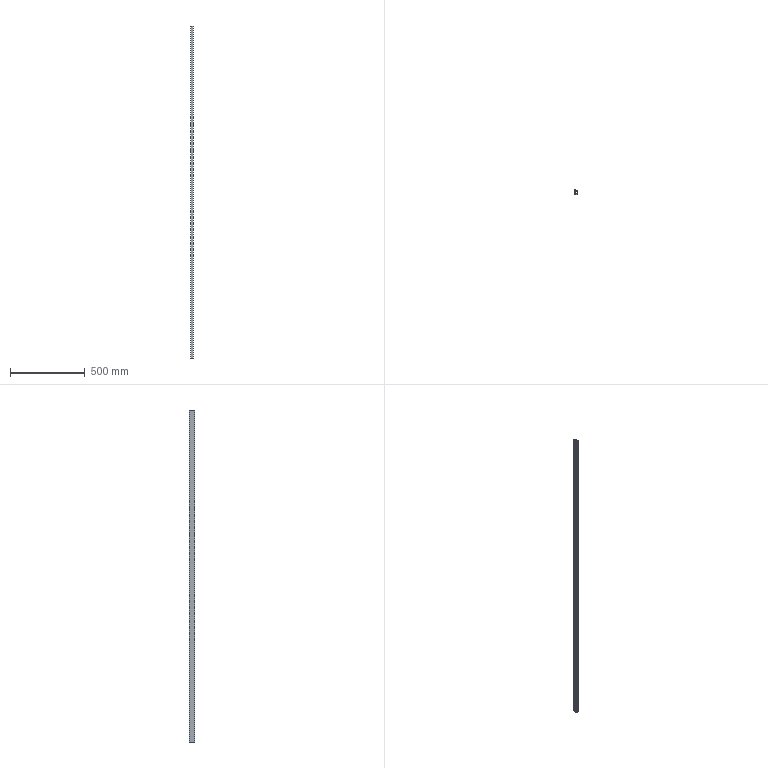Part | SolidWorks | features Extrusion 1 | 1 solid | 40 faces | box 14.605 x 34.798 x 2216 mm | volume 360474 mm3 | plane 23 | cylinder 17 | commonest cylinder face diameters 0.24 x4 0.2 x3 0.4 x2 0.5 x2 1 x2 1.2 x2
STEP:
#1=CARTESIAN_POINT('',(5.7,32.998,1108.));
#2=VERTEX_POINT('',#1);
#3=CARTESIAN_POINT('',(5.8,32.898,1108.));
#4=VERTEX_POINT('',#3);
#5=CARTESIAN_POINT('',(5.8,32.998,1108.));
#6=DIRECTION('',(0.,0.,1.));
#7=DIRECTION('',(1.,0.,0.));
#8=AXIS2_PLACEMENT_3D('',#5,#6,#7);
#9=CIRCLE('',#8,0.1);
#10=EDGE_CURVE('',#2,#4,#9,.T.);
#11=ORIENTED_EDGE('',*,*,#10,.F.);
#12=CARTESIAN_POINT('',(5.7,32.998,-1108.));
#13=VERTEX_POINT('',#12);
#14=CARTESIAN_POINT('',(5.7,32.998,1108.));
#15=DIRECTION('',(0.,0.,-1.));
#16=VECTOR('',#15,1000.);
#17=LINE('',#14,#16);
#18=EDGE_CURVE('',#2,#13,#17,.T.);
#19=ORIENTED_EDGE('',*,*,#18,.T.);
#20=CARTESIAN_POINT('',(5.8,32.898,-1108.));
#21=VERTEX_POINT('',#20);
#22=CARTESIAN_POINT('',(5.8,32.998,-1108.));
#23=DIRECTION('',(0.,0.,1.));
#24=DIRECTION('',(1.,0.,0.));
#25=AXIS2_PLACEMENT_3D('',#22,#23,#24);
#26=CIRCLE('',#25,0.1);
#27=EDGE_CURVE('',#13,#21,#26,.T.);
#28=ORIENTED_EDGE('',*,*,#27,.T.);
#29=CARTESIAN_POINT('',(5.8,32.898,1108.));
#30=DIRECTION('',(0.,0.,-1.));
#31=VECTOR('',#30,1000.);
#32=LINE('',#29,#31);
#33=EDGE_CURVE('',#4,#21,#32,.T.);
#34=ORIENTED_EDGE('',*,*,#33,.F.);
#35=EDGE_LOOP('',(#11,#19,#28,#34));
#36=FACE_OUTER_BOUND('',#35,.T.);
#37=CARTESIAN_POINT('',(5.8,32.998,1108.));
#38=DIRECTION('',(0.,0.,-1.));
#39=DIRECTION('',(-1.,0.,0.));
#40=AXIS2_PLACEMENT_3D('',#37,#38,#39);
#41=CYLINDRICAL_SURFACE('',#40,0.1);
#42=ADVANCED_FACE('',(#36),#41,.T.);
#43=CARTESIAN_POINT('',(1.75,10.,1108.));
#44=VERTEX_POINT('',#43);
#45=CARTESIAN_POINT('',(2.,10.25,1108.));
#46=VERTEX_POINT('',#45);
#47=CARTESIAN_POINT('',(2.,10.,1108.));
#48=DIRECTION('',(0.,0.,-1.));
#49=DIRECTION('',(1.,0.,0.));
#50=AXIS2_PLACEMENT_3D('',#47,#48,#49);
#51=CIRCLE('',#50,0.25);
#52=EDGE_CURVE('',#44,#46,#51,.T.);
#53=ORIENTED_EDGE('',*,*,#52,.F.);
#54=CARTESIAN_POINT('',(1.75,10.,-1108.));
#55=VERTEX_POINT('',#54);
#56=CARTESIAN_POINT('',(1.75,10.,1108.));
#57=DIRECTION('',(0.,0.,-1.));
#58=VECTOR('',#57,1000.);
#59=LINE('',#56,#58);
#60=EDGE_CURVE('',#44,#55,#59,.T.);
#61=ORIENTED_EDGE('',*,*,#60,.T.);
#62=CARTESIAN_POINT('',(2.,10.25,-1108.));
#63=VERTEX_POINT('',#62);
#64=CARTESIAN_POINT('',(2.,10.,-1108.));
#65=DIRECTION('',(0.,0.,-1.));
#66=DIRECTION('',(1.,0.,0.));
#67=AXIS2_PLACEMENT_3D('',#64,#65,#66);
#68=CIRCLE('',#67,0.25);
#69=EDGE_CURVE('',#55,#63,#68,.T.);
#70=ORIENTED_EDGE('',*,*,#69,.T.);
#71=CARTESIAN_POINT('',(2.,10.25,1108.));
#72=DIRECTION('',(0.,0.,-1.));
#73=VECTOR('',#72,1000.);
#74=LINE('',#71,#73);
#75=EDGE_CURVE('',#46,#63,#74,.T.);
#76=ORIENTED_EDGE('',*,*,#75,.F.);
#77=EDGE_LOOP('',(#53,#61,#70,#76));
#78=FACE_OUTER_BOUND('',#77,.T.);
#79=CARTESIAN_POINT('',(2.,10.,1108.));
#80=DIRECTION('',(0.,0.,-1.));
#81=DIRECTION('',(-1.,0.,0.));
#82=AXIS2_PLACEMENT_3D('',#79,#80,#81);
#83=CYLINDRICAL_SURFACE('',#82,0.25);
#84=ADVANCED_FACE('',(#78),#83,.F.);
#85=CARTESIAN_POINT('',(14.605,7.029,-1108.));
#86=VERTEX_POINT('',#85);
#87=CARTESIAN_POINT('',(14.485,7.149,-1108.));
#88=VERTEX_POINT('',#87);
#89=CARTESIAN_POINT('',(14.485,7.029,-1108.));
#90=DIRECTION('',(0.,0.,1.));
#91=DIRECTION('',(1.,0.,0.));
#92=AXIS2_PLACEMENT_3D('',#89,#90,#91);
#93=CIRCLE('',#92,0.12);
#94=EDGE_CURVE('',#86,#88,#93,.T.);
#95=ORIENTED_EDGE('',*,*,#94,.T.);
#96=CARTESIAN_POINT('',(14.485,7.149,1108.));
#97=VERTEX_POINT('',#96);
#98=CARTESIAN_POINT('',(14.485,7.149,1108.));
#99=DIRECTION('',(0.,0.,-1.));
#100=VECTOR('',#99,1000.);
#101=LINE('',#98,#100);
#102=EDGE_CURVE('',#97,#88,#101,.T.);
#103=ORIENTED_EDGE('',*,*,#102,.F.);
#104=CARTESIAN_POINT('',(14.605,7.029,1108.));
#105=VERTEX_POINT('',#104);
#106=CARTESIAN_POINT('',(14.485,7.029,1108.));
#107=DIRECTION('',(0.,0.,1.));
#108=DIRECTION('',(1.,0.,0.));
#109=AXIS2_PLACEMENT_3D('',#106,#107,#108);
#110=CIRCLE('',#109,0.12);
#111=EDGE_CURVE('',#105,#97,#110,.T.);
#112=ORIENTED_EDGE('',*,*,#111,.F.);
#113=CARTESIAN_POINT('',(14.605,7.029,1108.));
#114=DIRECTION('',(0.,0.,-1.));
#115=VECTOR('',#114,1000.);
#116=LINE('',#113,#115);
#117=EDGE_CURVE('',#105,#86,#116,.T.);
#118=ORIENTED_EDGE('',*,*,#117,.T.);
#119=EDGE_LOOP('',(#95,#103,#112,#118));
#120=FACE_OUTER_BOUND('',#119,.T.);
#121=CARTESIAN_POINT('',(14.485,7.029,1108.));
#122=DIRECTION('',(0.,0.,-1.));
#123=DIRECTION('',(-1.,0.,0.));
#124=AXIS2_PLACEMENT_3D('',#121,#122,#123);
#125=CYLINDRICAL_SURFACE('',#124,0.12);
#126=ADVANCED_FACE('',(#120),#125,.T.);
#127=CARTESIAN_POINT('',(13.705,7.149,-1108.));
#128=VERTEX_POINT('',#127);
#129=CARTESIAN_POINT('',(14.485,7.149,-1108.));
#130=DIRECTION('',(-1.,0.,0.));
#131=VECTOR('',#130,1000.);
#132=LINE('',#129,#131);
#133=EDGE_CURVE('',#88,#128,#132,.T.);
#134=ORIENTED_EDGE('',*,*,#133,.T.);
#135=CARTESIAN_POINT('',(13.705,7.149,1108.));
#136=VERTEX_POINT('',#135);
#137=CARTESIAN_POINT('',(13.705,7.149,1108.));
#138=DIRECTION('',(0.,0.,-1.));
#139=VECTOR('',#138,1000.);
#140=LINE('',#137,#139);
#141=EDGE_CURVE('',#136,#128,#140,.T.);
#142=ORIENTED_EDGE('',*,*,#141,.F.);
#143=CARTESIAN_POINT('',(14.485,7.149,1108.));
#144=DIRECTION('',(-1.,0.,0.));
#145=VECTOR('',#144,1000.);
#146=LINE('',#143,#145);
#147=EDGE_CURVE('',#97,#136,#146,.T.);
#148=ORIENTED_EDGE('',*,*,#147,.F.);
#149=ORIENTED_EDGE('',*,*,#102,.T.);
#150=EDGE_LOOP('',(#134,#142,#148,#149));
#151=FACE_OUTER_BOUND('',#150,.T.);
#152=CARTESIAN_POINT('',(14.485,7.149,1108.));
#153=DIRECTION('',(0.,-1.,0.));
#154=DIRECTION('',(0.,0.,-1.));
#155=AXIS2_PLACEMENT_3D('',#152,#153,#154);
#156=PLANE('',#155);
#157=ADVANCED_FACE('',(#151),#156,.F.);
#158=CARTESIAN_POINT('',(13.105,6.549,-1108.));
#159=VERTEX_POINT('',#158);
#160=CARTESIAN_POINT('',(13.705,6.549,-1108.));
#161=DIRECTION('',(0.,0.,1.));
#162=DIRECTION('',(1.,0.,0.));
#163=AXIS2_PLACEMENT_3D('',#160,#161,#162);
#164=CIRCLE('',#163,0.6);
#165=EDGE_CURVE('',#128,#159,#164,.T.);
#166=ORIENTED_EDGE('',*,*,#165,.T.);
#167=CARTESIAN_POINT('',(13.105,6.549,1108.));
#168=VERTEX_POINT('',#167);
#169=CARTESIAN_POINT('',(13.105,6.549,1108.));
#170=DIRECTION('',(0.,0.,-1.));
#171=VECTOR('',#170,1000.);
#172=LINE('',#169,#171);
#173=EDGE_CURVE('',#168,#159,#172,.T.);
#174=ORIENTED_EDGE('',*,*,#173,.F.);
#175=CARTESIAN_POINT('',(13.705,6.549,1108.));
#176=DIRECTION('',(0.,0.,1.));
#177=DIRECTION('',(1.,0.,0.));
#178=AXIS2_PLACEMENT_3D('',#175,#176,#177);
#179=CIRCLE('',#178,0.6);
#180=EDGE_CURVE('',#136,#168,#179,.T.);
#181=ORIENTED_EDGE('',*,*,#180,.F.);
#182=ORIENTED_EDGE('',*,*,#141,.T.);
#183=EDGE_LOOP('',(#166,#174,#181,#182));
#184=FACE_OUTER_BOUND('',#183,.T.);
#185=CARTESIAN_POINT('',(13.705,6.549,1108.));
#186=DIRECTION('',(0.,0.,-1.));
#187=DIRECTION('',(-1.,0.,0.));
#188=AXIS2_PLACEMENT_3D('',#185,#186,#187);
#189=CYLINDRICAL_SURFACE('',#188,0.6);
#190=ADVANCED_FACE('',(#184),#189,.T.);
#191=CARTESIAN_POINT('',(13.105,2.27,-1108.));
#192=VERTEX_POINT('',#191);
#193=CARTESIAN_POINT('',(13.105,6.549,-1108.));
#194=DIRECTION('',(0.,-1.,0.));
#195=VECTOR('',#194,1000.);
#196=LINE('',#193,#195);
#197=EDGE_CURVE('',#159,#192,#196,.T.);
#198=ORIENTED_EDGE('',*,*,#197,.T.);
#199=CARTESIAN_POINT('',(13.105,2.27,1108.));
#200=VERTEX_POINT('',#199);
#201=CARTESIAN_POINT('',(13.105,2.27,1108.));
#202=DIRECTION('',(0.,0.,-1.));
#203=VECTOR('',#202,1000.);
#204=LINE('',#201,#203);
#205=EDGE_CURVE('',#200,#192,#204,.T.);
#206=ORIENTED_EDGE('',*,*,#205,.F.);
#207=CARTESIAN_POINT('',(13.105,6.549,1108.));
#208=DIRECTION('',(0.,-1.,0.));
#209=VECTOR('',#208,1000.);
#210=LINE('',#207,#209);
#211=EDGE_CURVE('',#168,#200,#210,.T.);
#212=ORIENTED_EDGE('',*,*,#211,.F.);
#213=ORIENTED_EDGE('',*,*,#173,.T.);
#214=EDGE_LOOP('',(#198,#206,#212,#213));
#215=FACE_OUTER_BOUND('',#214,.T.);
#216=CARTESIAN_POINT('',(13.105,6.549,1108.));
#217=DIRECTION('',(1.,0.,0.));
#218=DIRECTION('',(0.,0.,-1.));
#219=AXIS2_PLACEMENT_3D('',#216,#217,#218);
#220=PLANE('',#219);
#221=ADVANCED_FACE('',(#215),#220,.F.);
#222=CARTESIAN_POINT('',(12.985,2.15,-1108.));
#223=VERTEX_POINT('',#222);
#224=CARTESIAN_POINT('',(12.985,2.27,-1108.));
#225=DIRECTION('',(0.,0.,-1.));
#226=DIRECTION('',(1.,0.,0.));
#227=AXIS2_PLACEMENT_3D('',#224,#225,#226);
#228=CIRCLE('',#227,0.12);
#229=EDGE_CURVE('',#192,#223,#228,.T.);
#230=ORIENTED_EDGE('',*,*,#229,.T.);
#231=CARTESIAN_POINT('',(12.985,2.15,1108.));
#232=VERTEX_POINT('',#231);
#233=CARTESIAN_POINT('',(12.985,2.15,1108.));
#234=DIRECTION('',(0.,0.,-1.));
#235=VECTOR('',#234,1000.);
#236=LINE('',#233,#235);
#237=EDGE_CURVE('',#232,#223,#236,.T.);
#238=ORIENTED_EDGE('',*,*,#237,.F.);
#239=CARTESIAN_POINT('',(12.985,2.27,1108.));
#240=DIRECTION('',(0.,0.,-1.));
#241=DIRECTION('',(1.,0.,0.));
#242=AXIS2_PLACEMENT_3D('',#239,#240,#241);
#243=CIRCLE('',#242,0.12);
#244=EDGE_CURVE('',#200,#232,#243,.T.);
#245=ORIENTED_EDGE('',*,*,#244,.F.);
#246=ORIENTED_EDGE('',*,*,#205,.T.);
#247=EDGE_LOOP('',(#230,#238,#245,#246));
#248=FACE_OUTER_BOUND('',#247,.T.);
#249=CARTESIAN_POINT('',(12.985,2.27,1108.));
#250=DIRECTION('',(0.,0.,-1.));
#251=DIRECTION('',(-1.,0.,0.));
#252=AXIS2_PLACEMENT_3D('',#249,#250,#251);
#253=CYLINDRICAL_SURFACE('',#252,0.12);
#254=ADVANCED_FACE('',(#248),#253,.F.);
#255=CARTESIAN_POINT('',(2.5,2.15,-1108.));
#256=VERTEX_POINT('',#255);
#257=CARTESIAN_POINT('',(12.985,2.15,-1108.));
#258=DIRECTION('',(-1.,0.00001466,0.));
#259=VECTOR('',#258,1000.);
#260=LINE('',#257,#259);
#261=EDGE_CURVE('',#223,#256,#260,.T.);
#262=ORIENTED_EDGE('',*,*,#261,.T.);
#263=CARTESIAN_POINT('',(2.5,2.15,1108.));
#264=VERTEX_POINT('',#263);
#265=CARTESIAN_POINT('',(2.5,2.15,1108.));
#266=DIRECTION('',(0.,0.,-1.));
#267=VECTOR('',#266,1000.);
#268=LINE('',#265,#267);
#269=EDGE_CURVE('',#264,#256,#268,.T.);
#270=ORIENTED_EDGE('',*,*,#269,.F.);
#271=CARTESIAN_POINT('',(12.985,2.15,1108.));
#272=DIRECTION('',(-1.,0.00001466,0.));
#273=VECTOR('',#272,1000.);
#274=LINE('',#271,#273);
#275=EDGE_CURVE('',#232,#264,#274,.T.);
#276=ORIENTED_EDGE('',*,*,#275,.F.);
#277=ORIENTED_EDGE('',*,*,#237,.T.);
#278=EDGE_LOOP('',(#262,#270,#276,#277));
#279=FACE_OUTER_BOUND('',#278,.T.);
#280=CARTESIAN_POINT('',(12.985,2.15,1108.));
#281=DIRECTION('',(-0.00001466,-1.,0.));
#282=DIRECTION('',(1.,-0.00001466,0.));
#283=AXIS2_PLACEMENT_3D('',#280,#281,#282);
#284=PLANE('',#283);
#285=ADVANCED_FACE('',(#279),#284,.F.);
#286=CARTESIAN_POINT('',(2.,2.65,-1108.));
#287=VERTEX_POINT('',#286);
#288=CARTESIAN_POINT('',(2.5,2.65,-1108.));
#289=DIRECTION('',(0.,0.,-1.));
#290=DIRECTION('',(1.,0.,0.));
#291=AXIS2_PLACEMENT_3D('',#288,#289,#290);
#292=CIRCLE('',#291,0.5);
#293=EDGE_CURVE('',#256,#287,#292,.T.);
#294=ORIENTED_EDGE('',*,*,#293,.T.);
#295=CARTESIAN_POINT('',(2.,2.65,1108.));
#296=VERTEX_POINT('',#295);
#297=CARTESIAN_POINT('',(2.,2.65,1108.));
#298=DIRECTION('',(0.,0.,-1.));
#299=VECTOR('',#298,1000.);
#300=LINE('',#297,#299);
#301=EDGE_CURVE('',#296,#287,#300,.T.);
#302=ORIENTED_EDGE('',*,*,#301,.F.);
#303=CARTESIAN_POINT('',(2.5,2.65,1108.));
#304=DIRECTION('',(0.,0.,-1.));
#305=DIRECTION('',(1.,0.,0.));
#306=AXIS2_PLACEMENT_3D('',#303,#304,#305);
#307=CIRCLE('',#306,0.5);
#308=EDGE_CURVE('',#264,#296,#307,.T.);
#309=ORIENTED_EDGE('',*,*,#308,.F.);
#310=ORIENTED_EDGE('',*,*,#269,.T.);
#311=EDGE_LOOP('',(#294,#302,#309,#310));
#312=FACE_OUTER_BOUND('',#311,.T.);
#313=CARTESIAN_POINT('',(2.5,2.65,1108.));
#314=DIRECTION('',(0.,0.,-1.));
#315=DIRECTION('',(-1.,0.,0.));
#316=AXIS2_PLACEMENT_3D('',#313,#314,#315);
#317=CYLINDRICAL_SURFACE('',#316,0.5);
#318=ADVANCED_FACE('',(#312),#317,.F.);
#319=CARTESIAN_POINT('',(2.,9.75,-1108.));
#320=VERTEX_POINT('',#319);
#321=CARTESIAN_POINT('',(2.,2.65,-1108.));
#322=DIRECTION('',(0.,1.,0.));
#323=VECTOR('',#322,1000.);
#324=LINE('',#321,#323);
#325=EDGE_CURVE('',#287,#320,#324,.T.);
#326=ORIENTED_EDGE('',*,*,#325,.T.);
#327=CARTESIAN_POINT('',(2.,9.75,1108.));
#328=VERTEX_POINT('',#327);
#329=CARTESIAN_POINT('',(2.,9.75,1108.));
#330=DIRECTION('',(0.,0.,-1.));
#331=VECTOR('',#330,1000.);
#332=LINE('',#329,#331);
#333=EDGE_CURVE('',#328,#320,#332,.T.);
#334=ORIENTED_EDGE('',*,*,#333,.F.);
#335=CARTESIAN_POINT('',(2.,2.65,1108.));
#336=DIRECTION('',(0.,1.,0.));
#337=VECTOR('',#336,1000.);
#338=LINE('',#335,#337);
#339=EDGE_CURVE('',#296,#328,#338,.T.);
#340=ORIENTED_EDGE('',*,*,#339,.F.);
#341=ORIENTED_EDGE('',*,*,#301,.T.);
#342=EDGE_LOOP('',(#326,#334,#340,#341));
#343=FACE_OUTER_BOUND('',#342,.T.);
#344=CARTESIAN_POINT('',(2.,2.65,1108.));
#345=DIRECTION('',(-1.,0.,0.));
#346=DIRECTION('',(0.,0.,1.));
#347=AXIS2_PLACEMENT_3D('',#344,#345,#346);
#348=PLANE('',#347);
#349=ADVANCED_FACE('',(#343),#348,.F.);
#350=ORIENTED_EDGE('',*,*,#60,.F.);
#351=CARTESIAN_POINT('',(2.,10.,1108.));
#352=DIRECTION('',(0.,0.,-1.));
#353=DIRECTION('',(1.,0.,0.));
#354=AXIS2_PLACEMENT_3D('',#351,#352,#353);
#355=CIRCLE('',#354,0.25);
#356=EDGE_CURVE('',#328,#44,#355,.T.);
#357=ORIENTED_EDGE('',*,*,#356,.F.);
#358=ORIENTED_EDGE('',*,*,#333,.T.);
#359=CARTESIAN_POINT('',(2.,10.,-1108.));
#360=DIRECTION('',(0.,0.,-1.));
#361=DIRECTION('',(1.,0.,0.));
#362=AXIS2_PLACEMENT_3D('',#359,#360,#361);
#363=CIRCLE('',#362,0.25);
#364=EDGE_CURVE('',#320,#55,#363,.T.);
#365=ORIENTED_EDGE('',*,*,#364,.T.);
#366=EDGE_LOOP('',(#350,#357,#358,#365));
#367=FACE_OUTER_BOUND('',#366,.T.);
#368=CARTESIAN_POINT('',(2.,10.,1108.));
#369=DIRECTION('',(0.,0.,-1.));
#370=DIRECTION('',(-1.,0.,0.));
#371=AXIS2_PLACEMENT_3D('',#368,#369,#370);
#372=CYLINDRICAL_SURFACE('',#371,0.25);
#373=ADVANCED_FACE('',(#367),#372,.F.);
#374=CARTESIAN_POINT('',(2.,17.35,-1108.));
#375=VERTEX_POINT('',#374);
#376=CARTESIAN_POINT('',(2.,10.25,-1108.));
#377=DIRECTION('',(0.,1.,0.));
#378=VECTOR('',#377,1000.);
#379=LINE('',#376,#378);
#380=EDGE_CURVE('',#63,#375,#379,.T.);
#381=ORIENTED_EDGE('',*,*,#380,.T.);
#382=CARTESIAN_POINT('',(2.,17.35,1108.));
#383=VERTEX_POINT('',#382);
#384=CARTESIAN_POINT('',(2.,17.35,1108.));
#385=DIRECTION('',(0.,0.,-1.));
#386=VECTOR('',#385,1000.);
#387=LINE('',#384,#386);
#388=EDGE_CURVE('',#383,#375,#387,.T.);
#389=ORIENTED_EDGE('',*,*,#388,.F.);
#390=CARTESIAN_POINT('',(2.,10.25,1108.));
#391=DIRECTION('',(0.,1.,0.));
#392=VECTOR('',#391,1000.);
#393=LINE('',#390,#392);
#394=EDGE_CURVE('',#46,#383,#393,.T.);
#395=ORIENTED_EDGE('',*,*,#394,.F.);
#396=ORIENTED_EDGE('',*,*,#75,.T.);
#397=EDGE_LOOP('',(#381,#389,#395,#396));
#398=FACE_OUTER_BOUND('',#397,.T.);
#399=CARTESIAN_POINT('',(2.,10.25,1108.));
#400=DIRECTION('',(-1.,0.,0.));
#401=DIRECTION('',(0.,0.,1.));
#402=AXIS2_PLACEMENT_3D('',#399,#400,#401);
#403=PLANE('',#402);
#404=ADVANCED_FACE('',(#398),#403,.F.);
#405=CARTESIAN_POINT('',(2.5,17.85,-1108.));
#406=VERTEX_POINT('',#405);
#407=CARTESIAN_POINT('',(2.5,17.35,-1108.));
#408=DIRECTION('',(0.,0.,-1.));
#409=DIRECTION('',(1.,0.,0.));
#410=AXIS2_PLACEMENT_3D('',#407,#408,#409);
#411=CIRCLE('',#410,0.5);
#412=EDGE_CURVE('',#375,#406,#411,.T.);
#413=ORIENTED_EDGE('',*,*,#412,.T.);
#414=CARTESIAN_POINT('',(2.5,17.85,1108.));
#415=VERTEX_POINT('',#414);
#416=CARTESIAN_POINT('',(2.5,17.85,1108.));
#417=DIRECTION('',(0.,0.,-1.));
#418=VECTOR('',#417,1000.);
#419=LINE('',#416,#418);
#420=EDGE_CURVE('',#415,#406,#419,.T.);
#421=ORIENTED_EDGE('',*,*,#420,.F.);
#422=CARTESIAN_POINT('',(2.5,17.35,1108.));
#423=DIRECTION('',(0.,0.,-1.));
#424=DIRECTION('',(1.,0.,0.));
#425=AXIS2_PLACEMENT_3D('',#422,#423,#424);
#426=CIRCLE('',#425,0.5);
#427=EDGE_CURVE('',#383,#415,#426,.T.);
#428=ORIENTED_EDGE('',*,*,#427,.F.);
#429=ORIENTED_EDGE('',*,*,#388,.T.);
#430=EDGE_LOOP('',(#413,#421,#428,#429));
#431=FACE_OUTER_BOUND('',#430,.T.);
#432=CARTESIAN_POINT('',(2.5,17.35,1108.));
#433=DIRECTION('',(0.,0.,-1.));
#434=DIRECTION('',(-1.,0.,0.));
#435=AXIS2_PLACEMENT_3D('',#432,#433,#434);
#436=CYLINDRICAL_SURFACE('',#435,0.5);
#437=ADVANCED_FACE('',(#431),#436,.F.);
#438=CARTESIAN_POINT('',(14.604,17.85,-1108.));
#439=VERTEX_POINT('',#438);
#440=CARTESIAN_POINT('',(2.5,17.85,-1108.));
#441=DIRECTION('',(1.,0.,0.));
#442=VECTOR('',#441,1000.);
#443=LINE('',#440,#442);
#444=EDGE_CURVE('',#406,#439,#443,.T.);
#445=ORIENTED_EDGE('',*,*,#444,.T.);
#446=CARTESIAN_POINT('',(14.604,17.85,1108.));
#447=VERTEX_POINT('',#446);
#448=CARTESIAN_POINT('',(14.604,17.85,1108.));
#449=DIRECTION('',(0.,0.,-1.));
#450=VECTOR('',#449,1000.);
#451=LINE('',#448,#450);
#452=EDGE_CURVE('',#447,#439,#451,.T.);
#453=ORIENTED_EDGE('',*,*,#452,.F.);
#454=CARTESIAN_POINT('',(2.5,17.85,1108.));
#455=DIRECTION('',(1.,0.,0.));
#456=VECTOR('',#455,1000.);
#457=LINE('',#454,#456);
#458=EDGE_CURVE('',#415,#447,#457,.T.);
#459=ORIENTED_EDGE('',*,*,#458,.F.);
#460=ORIENTED_EDGE('',*,*,#420,.T.);
#461=EDGE_LOOP('',(#445,#453,#459,#460));
#462=FACE_OUTER_BOUND('',#461,.T.);
#463=CARTESIAN_POINT('',(2.5,17.85,1108.));
#464=DIRECTION('',(0.,1.,0.));
#465=DIRECTION('',(0.,0.,1.));
#466=AXIS2_PLACEMENT_3D('',#463,#464,#465);
#467=PLANE('',#466);
#468=ADVANCED_FACE('',(#462),#467,.F.);
#469=CARTESIAN_POINT('',(14.604,23.83,-1108.));
#470=VERTEX_POINT('',#469);
#471=CARTESIAN_POINT('',(14.604,17.85,-1108.));
#472=DIRECTION('',(0.,1.,0.));
#473=VECTOR('',#472,1000.);
#474=LINE('',#471,#473);
#475=EDGE_CURVE('',#439,#470,#474,.T.);
#476=ORIENTED_EDGE('',*,*,#475,.T.);
#477=CARTESIAN_POINT('',(14.604,23.83,1108.));
#478=VERTEX_POINT('',#477);
#479=CARTESIAN_POINT('',(14.604,23.83,1108.));
#480=DIRECTION('',(0.,0.,-1.));
#481=VECTOR('',#480,1000.);
#482=LINE('',#479,#481);
#483=EDGE_CURVE('',#478,#470,#482,.T.);
#484=ORIENTED_EDGE('',*,*,#483,.F.);
#485=CARTESIAN_POINT('',(14.604,17.85,1108.));
#486=DIRECTION('',(0.,1.,0.));
#487=VECTOR('',#486,1000.);
#488=LINE('',#485,#487);
#489=EDGE_CURVE('',#447,#478,#488,.T.);
#490=ORIENTED_EDGE('',*,*,#489,.F.);
#491=ORIENTED_EDGE('',*,*,#452,.T.);
#492=EDGE_LOOP('',(#476,#484,#490,#491));
#493=FACE_OUTER_BOUND('',#492,.T.);
#494=CARTESIAN_POINT('',(14.604,17.85,1108.));
#495=DIRECTION('',(-1.,0.,0.));
#496=DIRECTION('',(0.,0.,1.));
#497=AXIS2_PLACEMENT_3D('',#494,#495,#496);
#498=PLANE('',#497);
#499=ADVANCED_FACE('',(#493),#498,.F.);
#500=CARTESIAN_POINT('',(14.484,23.95,-1108.));
#501=VERTEX_POINT('',#500);
#502=CARTESIAN_POINT('',(14.484,23.83,-1108.));
#503=DIRECTION('',(0.,0.,1.));
#504=DIRECTION('',(1.,0.,0.));
#505=AXIS2_PLACEMENT_3D('',#502,#503,#504);
#506=CIRCLE('',#505,0.12);
#507=EDGE_CURVE('',#470,#501,#506,.T.);
#508=ORIENTED_EDGE('',*,*,#507,.T.);
#509=CARTESIAN_POINT('',(14.484,23.95,1108.));
#510=VERTEX_POINT('',#509);
#511=CARTESIAN_POINT('',(14.484,23.95,1108.));
#512=DIRECTION('',(0.,0.,-1.));
#513=VECTOR('',#512,1000.);
#514=LINE('',#511,#513);
#515=EDGE_CURVE('',#510,#501,#514,.T.);
#516=ORIENTED_EDGE('',*,*,#515,.F.);
#517=CARTESIAN_POINT('',(14.484,23.83,1108.));
#518=DIRECTION('',(0.,0.,1.));
#519=DIRECTION('',(1.,0.,0.));
#520=AXIS2_PLACEMENT_3D('',#517,#518,#519);
#521=CIRCLE('',#520,0.12);
#522=EDGE_CURVE('',#478,#510,#521,.T.);
#523=ORIENTED_EDGE('',*,*,#522,.F.);
#524=ORIENTED_EDGE('',*,*,#483,.T.);
#525=EDGE_LOOP('',(#508,#516,#523,#524));
#526=FACE_OUTER_BOUND('',#525,.T.);
#527=CARTESIAN_POINT('',(14.484,23.83,1108.));
#528=DIRECTION('',(0.,0.,-1.));
#529=DIRECTION('',(-1.,0.,0.));
#530=AXIS2_PLACEMENT_3D('',#527,#528,#529);
#531=CYLINDRICAL_SURFACE('',#530,0.12);
#532=ADVANCED_FACE('',(#526),#531,.T.);
#533=CARTESIAN_POINT('',(13.704,23.95,-1108.));
#534=VERTEX_POINT('',#533);
#535=CARTESIAN_POINT('',(14.484,23.95,-1108.));
#536=DIRECTION('',(-1.,0.,0.));
#537=VECTOR('',#536,1000.);
#538=LINE('',#535,#537);
#539=EDGE_CURVE('',#501,#534,#538,.T.);
#540=ORIENTED_EDGE('',*,*,#539,.T.);
#541=CARTESIAN_POINT('',(13.704,23.95,1108.));
#542=VERTEX_POINT('',#541);
#543=CARTESIAN_POINT('',(13.704,23.95,1108.));
#544=DIRECTION('',(0.,0.,-1.));
#545=VECTOR('',#544,1000.);
#546=LINE('',#543,#545);
#547=EDGE_CURVE('',#542,#534,#546,.T.);
#548=ORIENTED_EDGE('',*,*,#547,.F.);
#549=CARTESIAN_POINT('',(14.484,23.95,1108.));
#550=DIRECTION('',(-1.,0.,0.));
#551=VECTOR('',#550,1000.);
#552=LINE('',#549,#551);
#553=EDGE_CURVE('',#510,#542,#552,.T.);
#554=ORIENTED_EDGE('',*,*,#553,.F.);
#555=ORIENTED_EDGE('',*,*,#515,.T.);
#556=EDGE_LOOP('',(#540,#548,#554,#555));
#557=FACE_OUTER_BOUND('',#556,.T.);
#558=CARTESIAN_POINT('',(14.484,23.95,1108.));
#559=DIRECTION('',(0.,-1.,0.));
#560=DIRECTION('',(0.,0.,-1.));
#561=AXIS2_PLACEMENT_3D('',#558,#559,#560);
#562=PLANE('',#561);
#563=ADVANCED_FACE('',(#557),#562,.F.);
#564=CARTESIAN_POINT('',(13.104,23.35,-1108.));
#565=VERTEX_POINT('',#564);
#566=CARTESIAN_POINT('',(13.704,23.35,-1108.));
#567=DIRECTION('',(0.,0.,1.));
#568=DIRECTION('',(1.,0.,0.));
#569=AXIS2_PLACEMENT_3D('',#566,#567,#568);
#570=CIRCLE('',#569,0.6);
#571=EDGE_CURVE('',#534,#565,#570,.T.);
#572=ORIENTED_EDGE('',*,*,#571,.T.);
#573=CARTESIAN_POINT('',(13.104,23.35,1108.));
#574=VERTEX_POINT('',#573);
#575=CARTESIAN_POINT('',(13.104,23.35,1108.));
#576=DIRECTION('',(0.,0.,-1.));
#577=VECTOR('',#576,1000.);
#578=LINE('',#575,#577);
#579=EDGE_CURVE('',#574,#565,#578,.T.);
#580=ORIENTED_EDGE('',*,*,#579,.F.);
#581=CARTESIAN_POINT('',(13.704,23.35,1108.));
#582=DIRECTION('',(0.,0.,1.));
#583=DIRECTION('',(1.,0.,0.));
#584=AXIS2_PLACEMENT_3D('',#581,#582,#583);
#585=CIRCLE('',#584,0.6);
#586=EDGE_CURVE('',#542,#574,#585,.T.);
#587=ORIENTED_EDGE('',*,*,#586,.F.);
#588=ORIENTED_EDGE('',*,*,#547,.T.);
#589=EDGE_LOOP('',(#572,#580,#587,#588));
#590=FACE_OUTER_BOUND('',#589,.T.);
#591=CARTESIAN_POINT('',(13.704,23.35,1108.));
#592=DIRECTION('',(0.,0.,-1.));
#593=DIRECTION('',(-1.,0.,0.));
#594=AXIS2_PLACEMENT_3D('',#591,#592,#593);
#595=CYLINDRICAL_SURFACE('',#594,0.6);
#596=ADVANCED_FACE('',(#590),#595,.T.);
#597=CARTESIAN_POINT('',(13.104,19.47,-1108.));
#598=VERTEX_POINT('',#597);
#599=CARTESIAN_POINT('',(13.104,23.35,-1108.));
#600=DIRECTION('',(0.,-1.,0.));
#601=VECTOR('',#600,1000.);
#602=LINE('',#599,#601);
#603=EDGE_CURVE('',#565,#598,#602,.T.);
#604=ORIENTED_EDGE('',*,*,#603,.T.);
#605=CARTESIAN_POINT('',(13.104,19.47,1108.));
#606=VERTEX_POINT('',#605);
#607=CARTESIAN_POINT('',(13.104,19.47,1108.));
#608=DIRECTION('',(0.,0.,-1.));
#609=VECTOR('',#608,1000.);
#610=LINE('',#607,#609);
#611=EDGE_CURVE('',#606,#598,#610,.T.);
#612=ORIENTED_EDGE('',*,*,#611,.F.);
#613=CARTESIAN_POINT('',(13.104,23.35,1108.));
#614=DIRECTION('',(0.,-1.,0.));
#615=VECTOR('',#614,1000.);
#616=LINE('',#613,#615);
#617=EDGE_CURVE('',#574,#606,#616,.T.);
#618=ORIENTED_EDGE('',*,*,#617,.F.);
#619=ORIENTED_EDGE('',*,*,#579,.T.);
#620=EDGE_LOOP('',(#604,#612,#618,#619));
#621=FACE_OUTER_BOUND('',#620,.T.);
#622=CARTESIAN_POINT('',(13.104,23.35,1108.));
#623=DIRECTION('',(1.,0.,0.));
#624=DIRECTION('',(0.,0.,-1.));
#625=AXIS2_PLACEMENT_3D('',#622,#623,#624);
#626=PLANE('',#625);
#627=ADVANCED_FACE('',(#621),#626,.F.);
#628=CARTESIAN_POINT('',(12.984,19.35,-1108.));
#629=VERTEX_POINT('',#628);
#630=CARTESIAN_POINT('',(12.984,19.47,-1108.));
#631=DIRECTION('',(0.,0.,-1.));
#632=DIRECTION('',(1.,0.,0.));
#633=AXIS2_PLACEMENT_3D('',#630,#631,#632);
#634=CIRCLE('',#633,0.12);
#635=EDGE_CURVE('',#598,#629,#634,.T.);
#636=ORIENTED_EDGE('',*,*,#635,.T.);
#637=CARTESIAN_POINT('',(12.984,19.35,1108.));
#638=VERTEX_POINT('',#637);
#639=CARTESIAN_POINT('',(12.984,19.35,1108.));
#640=DIRECTION('',(0.,0.,-1.));
#641=VECTOR('',#640,1000.);
#642=LINE('',#639,#641);
#643=EDGE_CURVE('',#638,#629,#642,.T.);
#644=ORIENTED_EDGE('',*,*,#643,.F.);
#645=CARTESIAN_POINT('',(12.984,19.47,1108.));
#646=DIRECTION('',(0.,0.,-1.));
#647=DIRECTION('',(1.,0.,0.));
#648=AXIS2_PLACEMENT_3D('',#645,#646,#647);
#649=CIRCLE('',#648,0.12);
#650=EDGE_CURVE('',#606,#638,#649,.T.);
#651=ORIENTED_EDGE('',*,*,#650,.F.);
#652=ORIENTED_EDGE('',*,*,#611,.T.);
#653=EDGE_LOOP('',(#636,#644,#651,#652));
#654=FACE_OUTER_BOUND('',#653,.T.);
#655=CARTESIAN_POINT('',(12.984,19.47,1108.));
#656=DIRECTION('',(0.,0.,-1.));
#657=DIRECTION('',(-1.,0.,0.));
#658=AXIS2_PLACEMENT_3D('',#655,#656,#657);
#659=CYLINDRICAL_SURFACE('',#658,0.12);
#660=ADVANCED_FACE('',(#654),#659,.F.);
#661=CARTESIAN_POINT('',(7.2,19.35,-1108.));
#662=VERTEX_POINT('',#661);
#663=CARTESIAN_POINT('',(12.984,19.35,-1108.));
#664=DIRECTION('',(-1.,0.,0.));
#665=VECTOR('',#664,1000.);
#666=LINE('',#663,#665);
#667=EDGE_CURVE('',#629,#662,#666,.T.);
#668=ORIENTED_EDGE('',*,*,#667,.T.);
#669=CARTESIAN_POINT('',(7.2,19.35,1108.));
#670=VERTEX_POINT('',#669);
#671=CARTESIAN_POINT('',(7.2,19.35,1108.));
#672=DIRECTION('',(0.,0.,-1.));
#673=VECTOR('',#672,1000.);
#674=LINE('',#671,#673);
#675=EDGE_CURVE('',#670,#662,#674,.T.);
#676=ORIENTED_EDGE('',*,*,#675,.F.);
#677=CARTESIAN_POINT('',(12.984,19.35,1108.));
#678=DIRECTION('',(-1.,0.,0.));
#679=VECTOR('',#678,1000.);
#680=LINE('',#677,#679);
#681=EDGE_CURVE('',#638,#670,#680,.T.);
#682=ORIENTED_EDGE('',*,*,#681,.F.);
#683=ORIENTED_EDGE('',*,*,#643,.T.);
#684=EDGE_LOOP('',(#668,#676,#682,#683));
#685=FACE_OUTER_BOUND('',#684,.T.);
#686=CARTESIAN_POINT('',(12.984,19.35,1108.));
#687=DIRECTION('',(0.,-1.,0.));
#688=DIRECTION('',(0.,0.,-1.));
#689=AXIS2_PLACEMENT_3D('',#686,#687,#688);
#690=PLANE('',#689);
#691=ADVANCED_FACE('',(#685),#690,.F.);
#692=CARTESIAN_POINT('',(7.2,34.798,-1108.));
#693=VERTEX_POINT('',#692);
#694=CARTESIAN_POINT('',(7.2,19.35,-1108.));
#695=DIRECTION('',(0.,1.,0.));
#696=VECTOR('',#695,1000.);
#697=LINE('',#694,#696);
#698=EDGE_CURVE('',#662,#693,#697,.T.);
#699=ORIENTED_EDGE('',*,*,#698,.T.);
#700=CARTESIAN_POINT('',(7.2,34.798,1108.));
#701=VERTEX_POINT('',#700);
#702=CARTESIAN_POINT('',(7.2,34.798,1108.));
#703=DIRECTION('',(0.,0.,-1.));
#704=VECTOR('',#703,1000.);
#705=LINE('',#702,#704);
#706=EDGE_CURVE('',#701,#693,#705,.T.);
#707=ORIENTED_EDGE('',*,*,#706,.F.);
#708=CARTESIAN_POINT('',(7.2,19.35,1108.));
#709=DIRECTION('',(0.,1.,0.));
#710=VECTOR('',#709,1000.);
#711=LINE('',#708,#710);
#712=EDGE_CURVE('',#670,#701,#711,.T.);
#713=ORIENTED_EDGE('',*,*,#712,.F.);
#714=ORIENTED_EDGE('',*,*,#675,.T.);
#715=EDGE_LOOP('',(#699,#707,#713,#714));
#716=FACE_OUTER_BOUND('',#715,.T.);
#717=CARTESIAN_POINT('',(7.2,19.35,1108.));
#718=DIRECTION('',(-1.,0.,0.));
#719=DIRECTION('',(0.,0.,1.));
#720=AXIS2_PLACEMENT_3D('',#717,#718,#719);
#721=PLANE('',#720);
#722=ADVANCED_FACE('',(#716),#721,.F.);
#723=CARTESIAN_POINT('',(6.,34.798,-1108.));
#724=VERTEX_POINT('',#723);
#725=CARTESIAN_POINT('',(7.2,34.798,-1108.));
#726=DIRECTION('',(-1.,0.,0.));
#727=VECTOR('',#726,1000.);
#728=LINE('',#725,#727);
#729=EDGE_CURVE('',#693,#724,#728,.T.);
#730=ORIENTED_EDGE('',*,*,#729,.T.);
#731=CARTESIAN_POINT('',(6.,34.798,1108.));
#732=VERTEX_POINT('',#731);
#733=CARTESIAN_POINT('',(6.,34.798,1108.));
#734=DIRECTION('',(0.,0.,-1.));
#735=VECTOR('',#734,1000.);
#736=LINE('',#733,#735);
#737=EDGE_CURVE('',#732,#724,#736,.T.);
#738=ORIENTED_EDGE('',*,*,#737,.F.);
#739=CARTESIAN_POINT('',(7.2,34.798,1108.));
#740=DIRECTION('',(-1.,0.,0.));
#741=VECTOR('',#740,1000.);
#742=LINE('',#739,#741);
#743=EDGE_CURVE('',#701,#732,#742,.T.);
#744=ORIENTED_EDGE('',*,*,#743,.F.);
#745=ORIENTED_EDGE('',*,*,#706,.T.);
#746=EDGE_LOOP('',(#730,#738,#744,#745));
#747=FACE_OUTER_BOUND('',#746,.T.);
#748=CARTESIAN_POINT('',(7.2,34.798,1108.));
#749=DIRECTION('',(0.,-1.,0.));
#750=DIRECTION('',(0.,0.,-1.));
#751=AXIS2_PLACEMENT_3D('',#748,#749,#750);
#752=PLANE('',#751);
#753=ADVANCED_FACE('',(#747),#752,.F.);
#754=CARTESIAN_POINT('',(5.8,34.598,-1108.));
#755=VERTEX_POINT('',#754);
#756=CARTESIAN_POINT('',(6.,34.598,-1108.));
#757=DIRECTION('',(0.,0.,1.));
#758=DIRECTION('',(1.,0.,0.));
#759=AXIS2_PLACEMENT_3D('',#756,#757,#758);
#760=CIRCLE('',#759,0.2);
#761=EDGE_CURVE('',#724,#755,#760,.T.);
#762=ORIENTED_EDGE('',*,*,#761,.T.);
#763=CARTESIAN_POINT('',(5.8,34.598,1108.));
#764=VERTEX_POINT('',#763);
#765=CARTESIAN_POINT('',(5.8,34.598,1108.));
#766=DIRECTION('',(0.,0.,-1.));
#767=VECTOR('',#766,1000.);
#768=LINE('',#765,#767);
#769=EDGE_CURVE('',#764,#755,#768,.T.);
#770=ORIENTED_EDGE('',*,*,#769,.F.);
#771=CARTESIAN_POINT('',(6.,34.598,1108.));
#772=DIRECTION('',(0.,0.,1.));
#773=DIRECTION('',(1.,0.,0.));
#774=AXIS2_PLACEMENT_3D('',#771,#772,#773);
#775=CIRCLE('',#774,0.2);
#776=EDGE_CURVE('',#732,#764,#775,.T.);
#777=ORIENTED_EDGE('',*,*,#776,.F.);
#778=ORIENTED_EDGE('',*,*,#737,.T.);
#779=EDGE_LOOP('',(#762,#770,#777,#778));
#780=FACE_OUTER_BOUND('',#779,.T.);
#781=CARTESIAN_POINT('',(6.,34.598,1108.));
#782=DIRECTION('',(0.,0.,-1.));
#783=DIRECTION('',(-1.,0.,0.));
#784=AXIS2_PLACEMENT_3D('',#781,#782,#783);
#785=CYLINDRICAL_SURFACE('',#784,0.2);
#786=ADVANCED_FACE('',(#780),#785,.T.);
#787=CARTESIAN_POINT('',(5.8,33.098,-1108.));
#788=VERTEX_POINT('',#787);
#789=CARTESIAN_POINT('',(5.8,34.598,-1108.));
#790=DIRECTION('',(0.,-1.,0.));
#791=VECTOR('',#790,1000.);
#792=LINE('',#789,#791);
#793=EDGE_CURVE('',#755,#788,#792,.T.);
#794=ORIENTED_EDGE('',*,*,#793,.T.);
#795=CARTESIAN_POINT('',(5.8,33.098,1108.));
#796=VERTEX_POINT('',#795);
#797=CARTESIAN_POINT('',(5.8,33.098,1108.));
#798=DIRECTION('',(0.,0.,-1.));
#799=VECTOR('',#798,1000.);
#800=LINE('',#797,#799);
#801=EDGE_CURVE('',#796,#788,#800,.T.);
#802=ORIENTED_EDGE('',*,*,#801,.F.);
#803=CARTESIAN_POINT('',(5.8,34.598,1108.));
#804=DIRECTION('',(0.,-1.,0.));
#805=VECTOR('',#804,1000.);
#806=LINE('',#803,#805);
#807=EDGE_CURVE('',#764,#796,#806,.T.);
#808=ORIENTED_EDGE('',*,*,#807,.F.);
#809=ORIENTED_EDGE('',*,*,#769,.T.);
#810=EDGE_LOOP('',(#794,#802,#808,#809));
#811=FACE_OUTER_BOUND('',#810,.T.);
#812=CARTESIAN_POINT('',(5.8,34.598,1108.));
#813=DIRECTION('',(1.,0.,0.));
#814=DIRECTION('',(0.,0.,-1.));
#815=AXIS2_PLACEMENT_3D('',#812,#813,#814);
#816=PLANE('',#815);
#817=ADVANCED_FACE('',(#811),#816,.F.);
#818=ORIENTED_EDGE('',*,*,#18,.F.);
#819=CARTESIAN_POINT('',(5.8,32.998,1108.));
#820=DIRECTION('',(0.,0.,1.));
#821=DIRECTION('',(1.,0.,0.));
#822=AXIS2_PLACEMENT_3D('',#819,#820,#821);
#823=CIRCLE('',#822,0.1);
#824=EDGE_CURVE('',#796,#2,#823,.T.);
#825=ORIENTED_EDGE('',*,*,#824,.F.);
#826=ORIENTED_EDGE('',*,*,#801,.T.);
#827=CARTESIAN_POINT('',(5.8,32.998,-1108.));
#828=DIRECTION('',(0.,0.,1.));
#829=DIRECTION('',(1.,0.,0.));
#830=AXIS2_PLACEMENT_3D('',#827,#828,#829);
#831=CIRCLE('',#830,0.1);
#832=EDGE_CURVE('',#788,#13,#831,.T.);
#833=ORIENTED_EDGE('',*,*,#832,.T.);
#834=EDGE_LOOP('',(#818,#825,#826,#833));
#835=FACE_OUTER_BOUND('',#834,.T.);
#836=CARTESIAN_POINT('',(5.8,32.998,1108.));
#837=DIRECTION('',(0.,0.,-1.));
#838=DIRECTION('',(-1.,0.,0.));
#839=AXIS2_PLACEMENT_3D('',#836,#837,#838);
#840=CYLINDRICAL_SURFACE('',#839,0.1);
#841=ADVANCED_FACE('',(#835),#840,.T.);
#842=CARTESIAN_POINT('',(5.8,23.812,-1108.));
#843=VERTEX_POINT('',#842);
#844=CARTESIAN_POINT('',(5.8,32.898,-1108.));
#845=DIRECTION('',(0.,-1.,0.));
#846=VECTOR('',#845,1000.);
#847=LINE('',#844,#846);
#848=EDGE_CURVE('',#21,#843,#847,.T.);
#849=ORIENTED_EDGE('',*,*,#848,.T.);
#850=CARTESIAN_POINT('',(5.8,23.812,1108.));
#851=VERTEX_POINT('',#850);
#852=CARTESIAN_POINT('',(5.8,23.812,1108.));
#853=DIRECTION('',(0.,0.,-1.));
#854=VECTOR('',#853,1000.);
#855=LINE('',#852,#854);
#856=EDGE_CURVE('',#851,#843,#855,.T.);
#857=ORIENTED_EDGE('',*,*,#856,.F.);
#858=CARTESIAN_POINT('',(5.8,32.898,1108.));
#859=DIRECTION('',(0.,-1.,0.));
#860=VECTOR('',#859,1000.);
#861=LINE('',#858,#860);
#862=EDGE_CURVE('',#4,#851,#861,.T.);
#863=ORIENTED_EDGE('',*,*,#862,.F.);
#864=ORIENTED_EDGE('',*,*,#33,.T.);
#865=EDGE_LOOP('',(#849,#857,#863,#864));
#866=FACE_OUTER_BOUND('',#865,.T.);
#867=CARTESIAN_POINT('',(5.8,32.898,1108.));
#868=DIRECTION('',(1.,0.,0.));
#869=DIRECTION('',(0.,0.,-1.));
#870=AXIS2_PLACEMENT_3D('',#867,#868,#869);
#871=PLANE('',#870);
#872=ADVANCED_FACE('',(#866),#871,.F.);
#873=CARTESIAN_POINT('',(4.8,22.812,-1108.));
#874=VERTEX_POINT('',#873);
#875=CARTESIAN_POINT('',(4.8,23.812,-1108.));
#876=DIRECTION('',(0.,0.,-1.));
#877=DIRECTION('',(1.,0.,0.));
#878=AXIS2_PLACEMENT_3D('',#875,#876,#877);
#879=CIRCLE('',#878,1.);
#880=EDGE_CURVE('',#843,#874,#879,.T.);
#881=ORIENTED_EDGE('',*,*,#880,.T.);
#882=CARTESIAN_POINT('',(4.8,22.812,1108.));
#883=VERTEX_POINT('',#882);
#884=CARTESIAN_POINT('',(4.8,22.812,1108.));
#885=DIRECTION('',(0.,0.,-1.));
#886=VECTOR('',#885,1000.);
#887=LINE('',#884,#886);
#888=EDGE_CURVE('',#883,#874,#887,.T.);
#889=ORIENTED_EDGE('',*,*,#888,.F.);
#890=CARTESIAN_POINT('',(4.8,23.812,1108.));
#891=DIRECTION('',(0.,0.,-1.));
#892=DIRECTION('',(1.,0.,0.));
#893=AXIS2_PLACEMENT_3D('',#890,#891,#892);
#894=CIRCLE('',#893,1.);
#895=EDGE_CURVE('',#851,#883,#894,.T.);
#896=ORIENTED_EDGE('',*,*,#895,.F.);
#897=ORIENTED_EDGE('',*,*,#856,.T.);
#898=EDGE_LOOP('',(#881,#889,#896,#897));
#899=FACE_OUTER_BOUND('',#898,.T.);
#900=CARTESIAN_POINT('',(4.8,23.812,1108.));
#901=DIRECTION('',(0.,0.,-1.));
#902=DIRECTION('',(-1.,0.,0.));
#903=AXIS2_PLACEMENT_3D('',#900,#901,#902);
#904=CYLINDRICAL_SURFACE('',#903,1.);
#905=ADVANCED_FACE('',(#899),#904,.F.);
#906=CARTESIAN_POINT('',(2.8,22.812,-1108.));
#907=VERTEX_POINT('',#906);
#908=CARTESIAN_POINT('',(4.8,22.812,-1108.));
#909=DIRECTION('',(-1.,0.,0.));
#910=VECTOR('',#909,1000.);
#911=LINE('',#908,#910);
#912=EDGE_CURVE('',#874,#907,#911,.T.);
#913=ORIENTED_EDGE('',*,*,#912,.T.);
#914=CARTESIAN_POINT('',(2.8,22.812,1108.));
#915=VERTEX_POINT('',#914);
#916=CARTESIAN_POINT('',(2.8,22.812,1108.));
#917=DIRECTION('',(0.,0.,-1.));
#918=VECTOR('',#917,1000.);
#919=LINE('',#916,#918);
#920=EDGE_CURVE('',#915,#907,#919,.T.);
#921=ORIENTED_EDGE('',*,*,#920,.F.);
#922=CARTESIAN_POINT('',(4.8,22.812,1108.));
#923=DIRECTION('',(-1.,0.,0.));
#924=VECTOR('',#923,1000.);
#925=LINE('',#922,#924);
#926=EDGE_CURVE('',#883,#915,#925,.T.);
#927=ORIENTED_EDGE('',*,*,#926,.F.);
#928=ORIENTED_EDGE('',*,*,#888,.T.);
#929=EDGE_LOOP('',(#913,#921,#927,#928));
#930=FACE_OUTER_BOUND('',#929,.T.);
#931=CARTESIAN_POINT('',(4.8,22.812,1108.));
#932=DIRECTION('',(0.,-1.,0.));
#933=DIRECTION('',(0.,0.,-1.));
#934=AXIS2_PLACEMENT_3D('',#931,#932,#933);
#935=PLANE('',#934);
#936=ADVANCED_FACE('',(#930),#935,.F.);
#937=CARTESIAN_POINT('',(1.8,23.812,-1108.));
#938=VERTEX_POINT('',#937);
#939=CARTESIAN_POINT('',(2.8,23.812,-1108.));
#940=DIRECTION('',(0.,0.,-1.));
#941=DIRECTION('',(1.,0.,0.));
#942=AXIS2_PLACEMENT_3D('',#939,#940,#941);
#943=CIRCLE('',#942,1.);
#944=EDGE_CURVE('',#907,#938,#943,.T.);
#945=ORIENTED_EDGE('',*,*,#944,.T.);
#946=CARTESIAN_POINT('',(1.8,23.812,1108.));
#947=VERTEX_POINT('',#946);
#948=CARTESIAN_POINT('',(1.8,23.812,1108.));
#949=DIRECTION('',(0.,0.,-1.));
#950=VECTOR('',#949,1000.);
#951=LINE('',#948,#950);
#952=EDGE_CURVE('',#947,#938,#951,.T.);
#953=ORIENTED_EDGE('',*,*,#952,.F.);
#954=CARTESIAN_POINT('',(2.8,23.812,1108.));
#955=DIRECTION('',(0.,0.,-1.));
#956=DIRECTION('',(1.,0.,0.));
#957=AXIS2_PLACEMENT_3D('',#954,#955,#956);
#958=CIRCLE('',#957,1.);
#959=EDGE_CURVE('',#915,#947,#958,.T.);
#960=ORIENTED_EDGE('',*,*,#959,.F.);
#961=ORIENTED_EDGE('',*,*,#920,.T.);
#962=EDGE_LOOP('',(#945,#953,#960,#961));
#963=FACE_OUTER_BOUND('',#962,.T.);
#964=CARTESIAN_POINT('',(2.8,23.812,1108.));
#965=DIRECTION('',(0.,0.,-1.));
#966=DIRECTION('',(-1.,0.,0.));
#967=AXIS2_PLACEMENT_3D('',#964,#965,#966);
#968=CYLINDRICAL_SURFACE('',#967,1.);
#969=ADVANCED_FACE('',(#963),#968,.F.);
#970=CARTESIAN_POINT('',(1.8,32.898,-1108.));
#971=VERTEX_POINT('',#970);
#972=CARTESIAN_POINT('',(1.8,23.812,-1108.));
#973=DIRECTION('',(0.,1.,0.));
#974=VECTOR('',#973,1000.);
#975=LINE('',#972,#974);
#976=EDGE_CURVE('',#938,#971,#975,.T.);
#977=ORIENTED_EDGE('',*,*,#976,.T.);
#978=CARTESIAN_POINT('',(1.8,32.898,1108.));
#979=VERTEX_POINT('',#978);
#980=CARTESIAN_POINT('',(1.8,32.898,1108.));
#981=DIRECTION('',(0.,0.,-1.));
#982=VECTOR('',#981,1000.);
#983=LINE('',#980,#982);
#984=EDGE_CURVE('',#979,#971,#983,.T.);
#985=ORIENTED_EDGE('',*,*,#984,.F.);
#986=CARTESIAN_POINT('',(1.8,23.812,1108.));
#987=DIRECTION('',(0.,1.,0.));
#988=VECTOR('',#987,1000.);
#989=LINE('',#986,#988);
#990=EDGE_CURVE('',#947,#979,#989,.T.);
#991=ORIENTED_EDGE('',*,*,#990,.F.);
#992=ORIENTED_EDGE('',*,*,#952,.T.);
#993=EDGE_LOOP('',(#977,#985,#991,#992));
#994=FACE_OUTER_BOUND('',#993,.T.);
#995=CARTESIAN_POINT('',(1.8,23.812,1108.));
#996=DIRECTION('',(-1.,0.,0.));
#997=DIRECTION('',(0.,0.,1.));
#998=AXIS2_PLACEMENT_3D('',#995,#996,#997);
#999=PLANE('',#998);
#1000=ADVANCED_FACE('',(#994),#999,.F.);
#1001=CARTESIAN_POINT('',(1.8,33.098,-1108.));
#1002=VERTEX_POINT('',#1001);
#1003=CARTESIAN_POINT('',(1.8,32.998,-1108.));
#1004=DIRECTION('',(0.,0.,1.));
#1005=DIRECTION('',(1.,0.,0.));
#1006=AXIS2_PLACEMENT_3D('',#1003,#1004,#1005);
#1007=CIRCLE('',#1006,0.1);
#1008=EDGE_CURVE('',#971,#1002,#1007,.T.);
#1009=ORIENTED_EDGE('',*,*,#1008,.T.);
#1010=CARTESIAN_POINT('',(1.8,33.098,1108.));
#1011=VERTEX_POINT('',#1010);
#1012=CARTESIAN_POINT('',(1.8,33.098,1108.));
#1013=DIRECTION('',(0.,0.,-1.));
#1014=VECTOR('',#1013,1000.);
#1015=LINE('',#1012,#1014);
#1016=EDGE_CURVE('',#1011,#1002,#1015,.T.);
#1017=ORIENTED_EDGE('',*,*,#1016,.F.);
#1018=CARTESIAN_POINT('',(1.8,32.998,1108.));
#1019=DIRECTION('',(0.,0.,1.));
#1020=DIRECTION('',(1.,0.,0.));
#1021=AXIS2_PLACEMENT_3D('',#1018,#1019,#1020);
#1022=CIRCLE('',#1021,0.1);
#1023=EDGE_CURVE('',#979,#1011,#1022,.T.);
#1024=ORIENTED_EDGE('',*,*,#1023,.F.);
#1025=ORIENTED_EDGE('',*,*,#984,.T.);
#1026=EDGE_LOOP('',(#1009,#1017,#1024,#1025));
#1027=FACE_OUTER_BOUND('',#1026,.T.);
#1028=CARTESIAN_POINT('',(1.8,32.998,1108.));
#1029=DIRECTION('',(0.,0.,-1.));
#1030=DIRECTION('',(-1.,0.,0.));
#1031=AXIS2_PLACEMENT_3D('',#1028,#1029,#1030);
#1032=CYLINDRICAL_SURFACE('',#1031,0.1);
#1033=ADVANCED_FACE('',(#1027),#1032,.T.);
#1034=CARTESIAN_POINT('',(1.8,34.598,-1108.));
#1035=VERTEX_POINT('',#1034);
#1036=CARTESIAN_POINT('',(1.8,33.098,-1108.));
#1037=DIRECTION('',(0.,1.,0.));
#1038=VECTOR('',#1037,1000.);
#1039=LINE('',#1036,#1038);
#1040=EDGE_CURVE('',#1002,#1035,#1039,.T.);
#1041=ORIENTED_EDGE('',*,*,#1040,.T.);
#1042=CARTESIAN_POINT('',(1.8,34.598,1108.));
#1043=VERTEX_POINT('',#1042);
#1044=CARTESIAN_POINT('',(1.8,34.598,1108.));
#1045=DIRECTION('',(0.,0.,-1.));
#1046=VECTOR('',#1045,1000.);
#1047=LINE('',#1044,#1046);
#1048=EDGE_CURVE('',#1043,#1035,#1047,.T.);
#1049=ORIENTED_EDGE('',*,*,#1048,.F.);
#1050=CARTESIAN_POINT('',(1.8,33.098,1108.));
#1051=DIRECTION('',(0.,1.,0.));
#1052=VECTOR('',#1051,1000.);
#1053=LINE('',#1050,#1052);
#1054=EDGE_CURVE('',#1011,#1043,#1053,.T.);
#1055=ORIENTED_EDGE('',*,*,#1054,.F.);
#1056=ORIENTED_EDGE('',*,*,#1016,.T.);
#1057=EDGE_LOOP('',(#1041,#1049,#1055,#1056));
#1058=FACE_OUTER_BOUND('',#1057,.T.);
#1059=CARTESIAN_POINT('',(1.8,33.098,1108.));
#1060=DIRECTION('',(-1.,0.,0.));
#1061=DIRECTION('',(0.,0.,1.));
#1062=AXIS2_PLACEMENT_3D('',#1059,#1060,#1061);
#1063=PLANE('',#1062);
#1064=ADVANCED_FACE('',(#1058),#1063,.F.);
#1065=CARTESIAN_POINT('',(1.6,34.798,-1108.));
#1066=VERTEX_POINT('',#1065);
#1067=CARTESIAN_POINT('',(1.6,34.598,-1108.));
#1068=DIRECTION('',(0.,0.,1.));
#1069=DIRECTION('',(1.,0.,0.));
#1070=AXIS2_PLACEMENT_3D('',#1067,#1068,#1069);
#1071=CIRCLE('',#1070,0.2);
#1072=EDGE_CURVE('',#1035,#1066,#1071,.T.);
#1073=ORIENTED_EDGE('',*,*,#1072,.T.);
#1074=CARTESIAN_POINT('',(1.6,34.798,1108.));
#1075=VERTEX_POINT('',#1074);
#1076=CARTESIAN_POINT('',(1.6,34.798,1108.));
#1077=DIRECTION('',(0.,0.,-1.));
#1078=VECTOR('',#1077,1000.);
#1079=LINE('',#1076,#1078);
#1080=EDGE_CURVE('',#1075,#1066,#1079,.T.);
#1081=ORIENTED_EDGE('',*,*,#1080,.F.);
#1082=CARTESIAN_POINT('',(1.6,34.598,1108.));
#1083=DIRECTION('',(0.,0.,1.));
#1084=DIRECTION('',(1.,0.,0.));
#1085=AXIS2_PLACEMENT_3D('',#1082,#1083,#1084);
#1086=CIRCLE('',#1085,0.2);
#1087=EDGE_CURVE('',#1043,#1075,#1086,.T.);
#1088=ORIENTED_EDGE('',*,*,#1087,.F.);
#1089=ORIENTED_EDGE('',*,*,#1048,.T.);
#1090=EDGE_LOOP('',(#1073,#1081,#1088,#1089));
#1091=FACE_OUTER_BOUND('',#1090,.T.);
#1092=CARTESIAN_POINT('',(1.6,34.598,1108.));
#1093=DIRECTION('',(0.,0.,-1.));
#1094=DIRECTION('',(-1.,0.,0.));
#1095=AXIS2_PLACEMENT_3D('',#1092,#1093,#1094);
#1096=CYLINDRICAL_SURFACE('',#1095,0.2);
#1097=ADVANCED_FACE('',(#1091),#1096,.T.);
#1098=CARTESIAN_POINT('',(0.,34.798,-1108.));
#1099=VERTEX_POINT('',#1098);
#1100=CARTESIAN_POINT('',(1.6,34.798,-1108.));
#1101=DIRECTION('',(-1.,0.,0.));
#1102=VECTOR('',#1101,1000.);
#1103=LINE('',#1100,#1102);
#1104=EDGE_CURVE('',#1066,#1099,#1103,.T.);
#1105=ORIENTED_EDGE('',*,*,#1104,.T.);
#1106=CARTESIAN_POINT('',(0.,34.798,1108.));
#1107=VERTEX_POINT('',#1106);
#1108=CARTESIAN_POINT('',(0.,34.798,1108.));
#1109=DIRECTION('',(0.,0.,-1.));
#1110=VECTOR('',#1109,1000.);
#1111=LINE('',#1108,#1110);
#1112=EDGE_CURVE('',#1107,#1099,#1111,.T.);
#1113=ORIENTED_EDGE('',*,*,#1112,.F.);
#1114=CARTESIAN_POINT('',(1.6,34.798,1108.));
#1115=DIRECTION('',(-1.,0.,0.));
#1116=VECTOR('',#1115,1000.);
#1117=LINE('',#1114,#1116);
#1118=EDGE_CURVE('',#1075,#1107,#1117,.T.);
#1119=ORIENTED_EDGE('',*,*,#1118,.F.);
#1120=ORIENTED_EDGE('',*,*,#1080,.T.);
#1121=EDGE_LOOP('',(#1105,#1113,#1119,#1120));
#1122=FACE_OUTER_BOUND('',#1121,.T.);
#1123=CARTESIAN_POINT('',(1.6,34.798,1108.));
#1124=DIRECTION('',(0.,-1.,0.));
#1125=DIRECTION('',(0.,0.,-1.));
#1126=AXIS2_PLACEMENT_3D('',#1123,#1124,#1125);
#1127=PLANE('',#1126);
#1128=ADVANCED_FACE('',(#1122),#1127,.F.);
#1129=CARTESIAN_POINT('',(0.,0.,-1108.));
#1130=VERTEX_POINT('',#1129);
#1131=CARTESIAN_POINT('',(0.,34.798,-1108.));
#1132=DIRECTION('',(0.,-1.,0.));
#1133=VECTOR('',#1132,1000.);
#1134=LINE('',#1131,#1133);
#1135=EDGE_CURVE('',#1099,#1130,#1134,.T.);
#1136=ORIENTED_EDGE('',*,*,#1135,.T.);
#1137=CARTESIAN_POINT('',(0.,0.,1108.));
#1138=VERTEX_POINT('',#1137);
#1139=CARTESIAN_POINT('',(0.,0.,1108.));
#1140=DIRECTION('',(0.,0.,-1.));
#1141=VECTOR('',#1140,1000.);
#1142=LINE('',#1139,#1141);
#1143=EDGE_CURVE('',#1138,#1130,#1142,.T.);
#1144=ORIENTED_EDGE('',*,*,#1143,.F.);
#1145=CARTESIAN_POINT('',(0.,34.798,1108.));
#1146=DIRECTION('',(0.,-1.,0.));
#1147=VECTOR('',#1146,1000.);
#1148=LINE('',#1145,#1147);
#1149=EDGE_CURVE('',#1107,#1138,#1148,.T.);
#1150=ORIENTED_EDGE('',*,*,#1149,.F.);
#1151=ORIENTED_EDGE('',*,*,#1112,.T.);
#1152=EDGE_LOOP('',(#1136,#1144,#1150,#1151));
#1153=FACE_OUTER_BOUND('',#1152,.T.);
#1154=CARTESIAN_POINT('',(0.,34.798,1108.));
#1155=DIRECTION('',(1.,0.,0.));
#1156=DIRECTION('',(0.,0.,-1.));
#1157=AXIS2_PLACEMENT_3D('',#1154,#1155,#1156);
#1158=PLANE('',#1157);
#1159=ADVANCED_FACE('',(#1153),#1158,.F.);
#1160=CARTESIAN_POINT('',(14.6,0.,-1108.));
#1161=VERTEX_POINT('',#1160);
#1162=CARTESIAN_POINT('',(0.,0.,-1108.));
#1163=DIRECTION('',(1.,0.,0.));
#1164=VECTOR('',#1163,1000.);
#1165=LINE('',#1162,#1164);
#1166=EDGE_CURVE('',#1130,#1161,#1165,.T.);
#1167=ORIENTED_EDGE('',*,*,#1166,.T.);
#1168=CARTESIAN_POINT('',(14.6,0.,1108.));
#1169=VERTEX_POINT('',#1168);
#1170=CARTESIAN_POINT('',(14.6,0.,1108.));
#1171=DIRECTION('',(0.,0.,-1.));
#1172=VECTOR('',#1171,1000.);
#1173=LINE('',#1170,#1172);
#1174=EDGE_CURVE('',#1169,#1161,#1173,.T.);
#1175=ORIENTED_EDGE('',*,*,#1174,.F.);
#1176=CARTESIAN_POINT('',(0.,0.,1108.));
#1177=DIRECTION('',(1.,0.,0.));
#1178=VECTOR('',#1177,1000.);
#1179=LINE('',#1176,#1178);
#1180=EDGE_CURVE('',#1138,#1169,#1179,.T.);
#1181=ORIENTED_EDGE('',*,*,#1180,.F.);
#1182=ORIENTED_EDGE('',*,*,#1143,.T.);
#1183=EDGE_LOOP('',(#1167,#1175,#1181,#1182));
#1184=FACE_OUTER_BOUND('',#1183,.T.);
#1185=CARTESIAN_POINT('',(0.,0.,1108.));
#1186=DIRECTION('',(0.,1.,0.));
#1187=DIRECTION('',(0.,0.,1.));
#1188=AXIS2_PLACEMENT_3D('',#1185,#1186,#1187);
#1189=PLANE('',#1188);
#1190=ADVANCED_FACE('',(#1184),#1189,.F.);
#1191=CARTESIAN_POINT('',(14.6,0.,-1108.));
#1192=DIRECTION('',(0.0007044,1.,0.));
#1193=VECTOR('',#1192,1000.);
#1194=LINE('',#1191,#1193);
#1195=EDGE_CURVE('',#1161,#86,#1194,.T.);
#1196=ORIENTED_EDGE('',*,*,#1195,.T.);
#1197=ORIENTED_EDGE('',*,*,#117,.F.);
#1198=CARTESIAN_POINT('',(14.6,0.,1108.));
#1199=DIRECTION('',(0.0007044,1.,0.));
#1200=VECTOR('',#1199,1000.);
#1201=LINE('',#1198,#1200);
#1202=EDGE_CURVE('',#1169,#105,#1201,.T.);
#1203=ORIENTED_EDGE('',*,*,#1202,.F.);
#1204=ORIENTED_EDGE('',*,*,#1174,.T.);
#1205=EDGE_LOOP('',(#1196,#1197,#1203,#1204));
#1206=FACE_OUTER_BOUND('',#1205,.T.);
#1207=CARTESIAN_POINT('',(14.6,0.,1108.));
#1208=DIRECTION('',(-1.,0.0007044,0.));
#1209=DIRECTION('',(-0.0007044,-1.,0.));
#1210=AXIS2_PLACEMENT_3D('',#1207,#1208,#1209);
#1211=PLANE('',#1210);
#1212=ADVANCED_FACE('',(#1206),#1211,.F.);
#1213=ORIENTED_EDGE('',*,*,#111,.T.);
#1214=ORIENTED_EDGE('',*,*,#147,.T.);
#1215=ORIENTED_EDGE('',*,*,#180,.T.);
#1216=ORIENTED_EDGE('',*,*,#211,.T.);
#1217=ORIENTED_EDGE('',*,*,#244,.T.);
#1218=ORIENTED_EDGE('',*,*,#275,.T.);
#1219=ORIENTED_EDGE('',*,*,#308,.T.);
#1220=ORIENTED_EDGE('',*,*,#339,.T.);
#1221=ORIENTED_EDGE('',*,*,#356,.T.);
#1222=ORIENTED_EDGE('',*,*,#52,.T.);
#1223=ORIENTED_EDGE('',*,*,#394,.T.);
#1224=ORIENTED_EDGE('',*,*,#427,.T.);
#1225=ORIENTED_EDGE('',*,*,#458,.T.);
#1226=ORIENTED_EDGE('',*,*,#489,.T.);
#1227=ORIENTED_EDGE('',*,*,#522,.T.);
#1228=ORIENTED_EDGE('',*,*,#553,.T.);
#1229=ORIENTED_EDGE('',*,*,#586,.T.);
#1230=ORIENTED_EDGE('',*,*,#617,.T.);
#1231=ORIENTED_EDGE('',*,*,#650,.T.);
#1232=ORIENTED_EDGE('',*,*,#681,.T.);
#1233=ORIENTED_EDGE('',*,*,#712,.T.);
#1234=ORIENTED_EDGE('',*,*,#743,.T.);
#1235=ORIENTED_EDGE('',*,*,#776,.T.);
#1236=ORIENTED_EDGE('',*,*,#807,.T.);
#1237=ORIENTED_EDGE('',*,*,#824,.T.);
#1238=ORIENTED_EDGE('',*,*,#10,.T.);
#1239=ORIENTED_EDGE('',*,*,#862,.T.);
#1240=ORIENTED_EDGE('',*,*,#895,.T.);
#1241=ORIENTED_EDGE('',*,*,#926,.T.);
#1242=ORIENTED_EDGE('',*,*,#959,.T.);
#1243=ORIENTED_EDGE('',*,*,#990,.T.);
#1244=ORIENTED_EDGE('',*,*,#1023,.T.);
#1245=ORIENTED_EDGE('',*,*,#1054,.T.);
#1246=ORIENTED_EDGE('',*,*,#1087,.T.);
#1247=ORIENTED_EDGE('',*,*,#1118,.T.);
#1248=ORIENTED_EDGE('',*,*,#1149,.T.);
#1249=ORIENTED_EDGE('',*,*,#1180,.T.);
#1250=ORIENTED_EDGE('',*,*,#1202,.T.);
#1251=EDGE_LOOP('',(#1213,#1214,#1215,#1216,#1217,#1218,#1219,#1220,#1221,#1222,#1223,#1224,#1225,#1226,#1227,#1228,#1229,#1230,#1231,#1232,#1233,#1234,#1235,#1236,#1237,#1238,#1239,#1240,#1241,#1242,#1243,#1244,#1245,#1246,#1247,#1248,#1249,#1250));
#1252=FACE_OUTER_BOUND('',#1251,.T.);
#1253=CARTESIAN_POINT('',(14.485,7.029,1108.));
#1254=DIRECTION('',(0.,0.,1.));
#1255=DIRECTION('',(1.,0.,0.));
#1256=AXIS2_PLACEMENT_3D('',#1253,#1254,#1255);
#1257=PLANE('',#1256);
#1258=ADVANCED_FACE('',(#1252),#1257,.T.);
#1259=ORIENTED_EDGE('',*,*,#94,.F.);
#1260=ORIENTED_EDGE('',*,*,#1195,.F.);
#1261=ORIENTED_EDGE('',*,*,#1166,.F.);
#1262=ORIENTED_EDGE('',*,*,#1135,.F.);
#1263=ORIENTED_EDGE('',*,*,#1104,.F.);
#1264=ORIENTED_EDGE('',*,*,#1072,.F.);
#1265=ORIENTED_EDGE('',*,*,#1040,.F.);
#1266=ORIENTED_EDGE('',*,*,#1008,.F.);
#1267=ORIENTED_EDGE('',*,*,#976,.F.);
#1268=ORIENTED_EDGE('',*,*,#944,.F.);
#1269=ORIENTED_EDGE('',*,*,#912,.F.);
#1270=ORIENTED_EDGE('',*,*,#880,.F.);
#1271=ORIENTED_EDGE('',*,*,#848,.F.);
#1272=ORIENTED_EDGE('',*,*,#27,.F.);
#1273=ORIENTED_EDGE('',*,*,#832,.F.);
#1274=ORIENTED_EDGE('',*,*,#793,.F.);
#1275=ORIENTED_EDGE('',*,*,#761,.F.);
#1276=ORIENTED_EDGE('',*,*,#729,.F.);
#1277=ORIENTED_EDGE('',*,*,#698,.F.);
#1278=ORIENTED_EDGE('',*,*,#667,.F.);
#1279=ORIENTED_EDGE('',*,*,#635,.F.);
#1280=ORIENTED_EDGE('',*,*,#603,.F.);
#1281=ORIENTED_EDGE('',*,*,#571,.F.);
#1282=ORIENTED_EDGE('',*,*,#539,.F.);
#1283=ORIENTED_EDGE('',*,*,#507,.F.);
#1284=ORIENTED_EDGE('',*,*,#475,.F.);
#1285=ORIENTED_EDGE('',*,*,#444,.F.);
#1286=ORIENTED_EDGE('',*,*,#412,.F.);
#1287=ORIENTED_EDGE('',*,*,#380,.F.);
#1288=ORIENTED_EDGE('',*,*,#69,.F.);
#1289=ORIENTED_EDGE('',*,*,#364,.F.);
#1290=ORIENTED_EDGE('',*,*,#325,.F.);
#1291=ORIENTED_EDGE('',*,*,#293,.F.);
#1292=ORIENTED_EDGE('',*,*,#261,.F.);
#1293=ORIENTED_EDGE('',*,*,#229,.F.);
#1294=ORIENTED_EDGE('',*,*,#197,.F.);
#1295=ORIENTED_EDGE('',*,*,#165,.F.);
#1296=ORIENTED_EDGE('',*,*,#133,.F.);
#1297=EDGE_LOOP('',(#1259,#1260,#1261,#1262,#1263,#1264,#1265,#1266,#1267,#1268,#1269,#1270,#1271,#1272,#1273,#1274,#1275,#1276,#1277,#1278,#1279,#1280,#1281,#1282,#1283,#1284,#1285,#1286,#1287,#1288,#1289,#1290,#1291,#1292,#1293,#1294,#1295,#1296));
#1298=FACE_OUTER_BOUND('',#1297,.T.);
#1299=CARTESIAN_POINT('',(14.485,7.029,-1108.));
#1300=DIRECTION('',(0.,0.,1.));
#1301=DIRECTION('',(1.,0.,0.));
#1302=AXIS2_PLACEMENT_3D('',#1299,#1300,#1301);
#1303=PLANE('',#1302);
#1304=ADVANCED_FACE('',(#1298),#1303,.F.);
#1305=CLOSED_SHELL('',(#42,#84,#126,#157,#190,#221,#254,#285,#318,#349,#373,#404,#437,#468,#499,#532,#563,#596,#627,#660,#691,#722,#753,#786,#817,#841,#872,#905,#936,#969,#1000,#1033,#1064,#1097,#1128,#1159,#1190,#1212,#1258,#1304));
#1306=MANIFOLD_SOLID_BREP('',#1305);
#1307=CARTESIAN_POINT('',(0.,0.,0.));
#1308=DIRECTION('',(0.,0.,1.));
#1309=DIRECTION('',(1.,0.,0.));
#1310=AXIS2_PLACEMENT_3D('',#1307,#1308,#1309);
#1311=(LENGTH_UNIT()NAMED_UNIT(*)SI_UNIT(.MILLI.,.METRE.));
#1312=UNCERTAINTY_MEASURE_WITH_UNIT(LENGTH_MEASURE(0.00001),#1311,'','');
#1313=(NAMED_UNIT(*)PLANE_ANGLE_UNIT()SI_UNIT($,.RADIAN.));
#1314=(NAMED_UNIT(*)SI_UNIT($,.STERADIAN.)SOLID_ANGLE_UNIT());
#1315=(GEOMETRIC_REPRESENTATION_CONTEXT(3)GLOBAL_UNCERTAINTY_ASSIGNED_CONTEXT((#1312))GLOBAL_UNIT_ASSIGNED_CONTEXT((#1311,#1313,#1314))REPRESENTATION_CONTEXT('',''));
#1316=ADVANCED_BREP_SHAPE_REPRESENTATION('',(#1306,#1310),#1315);